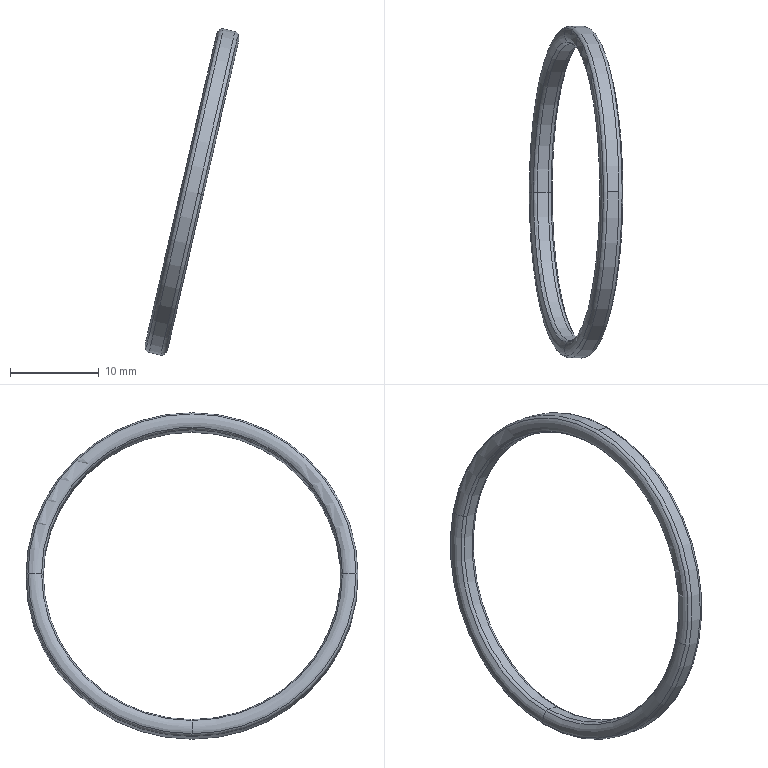Part | SolidWorks | features BaseBody 1 | 1 solid | 19 faces | box 10.587 x 37.5 x 36.875 mm | volume 507.842 mm3 | torus 15 | cylinder 4 | commonest cylinder face diameters 33.6 x2 37.5 x2
STEP:
#1=CARTESIAN_POINT('',(1987.878,-194.526,844.998));
#2=VERTEX_POINT('',#1);
#3=CARTESIAN_POINT('',(1983.731,-176.,826.943));
#4=VERTEX_POINT('',#3);
#5=CARTESIAN_POINT('',(1987.878,-176.,844.998));
#6=DIRECTION('',(0.9746,0.,-0.2239));
#7=DIRECTION('',(0.,-1.,0.));
#8=AXIS2_PLACEMENT_3D('',#5,#6,#7);
#9=CIRCLE('',#8,18.526);
#10=EDGE_CURVE('',#2,#4,#9,.T.);
#11=ORIENTED_EDGE('',*,*,#10,.F.);
#12=CARTESIAN_POINT('',(1987.472,-194.75,845.091));
#13=VERTEX_POINT('',#12);
#14=CARTESIAN_POINT('',(1987.472,-194.25,845.091));
#15=DIRECTION('',(-0.2239,0.,-0.9746));
#16=DIRECTION('',(-0.9746,0.,0.2239));
#17=AXIS2_PLACEMENT_3D('',#14,#15,#16);
#18=CIRCLE('',#17,0.5);
#19=EDGE_CURVE('',#2,#13,#18,.T.);
#20=ORIENTED_EDGE('',*,*,#19,.T.);
#21=CARTESIAN_POINT('',(1983.274,-176.,826.817));
#22=VERTEX_POINT('',#21);
#23=CARTESIAN_POINT('',(1987.472,-176.,845.091));
#24=DIRECTION('',(-0.9746,0.,0.2239));
#25=DIRECTION('',(-0.2239,0.,-0.9746));
#26=AXIS2_PLACEMENT_3D('',#23,#24,#25);
#27=CIRCLE('',#26,18.75);
#28=EDGE_CURVE('',#22,#13,#27,.T.);
#29=ORIENTED_EDGE('',*,*,#28,.F.);
#30=CARTESIAN_POINT('',(1983.386,-176.,827.305));
#31=DIRECTION('',(0.,-1.,0.));
#32=DIRECTION('',(0.6899,0.,-0.7239));
#33=AXIS2_PLACEMENT_3D('',#30,#31,#32);
#34=CIRCLE('',#33,0.5);
#35=EDGE_CURVE('',#22,#4,#34,.T.);
#36=ORIENTED_EDGE('',*,*,#35,.T.);
#37=EDGE_LOOP('',(#11,#20,#29,#36));
#38=FACE_OUTER_BOUND('',#37,.T.);
#39=CARTESIAN_POINT('',(1987.472,-176.,845.091));
#40=DIRECTION('',(-0.9746,0.,0.2239));
#41=DIRECTION('',(0.,-1.,0.));
#42=AXIS2_PLACEMENT_3D('',#39,#40,#41);
#43=TOROIDAL_SURFACE('',#42,18.25,0.5);
#44=ADVANCED_FACE('',(#38),#43,.T.);
#45=CARTESIAN_POINT('',(1987.809,-159.013,845.014));
#46=VERTEX_POINT('',#45);
#47=CARTESIAN_POINT('',(1984.007,-176.,828.458));
#48=VERTEX_POINT('',#47);
#49=CARTESIAN_POINT('',(1987.809,-176.,845.014));
#50=DIRECTION('',(-0.9746,0.,0.2239));
#51=DIRECTION('',(0.,1.,0.));
#52=AXIS2_PLACEMENT_3D('',#49,#50,#51);
#53=CIRCLE('',#52,16.987);
#54=EDGE_CURVE('',#46,#48,#53,.T.);
#55=ORIENTED_EDGE('',*,*,#54,.T.);
#56=CARTESIAN_POINT('',(1982.829,-176.,827.889));
#57=DIRECTION('',(0.,1.,0.));
#58=DIRECTION('',(0.,0.,1.));
#59=AXIS2_PLACEMENT_3D('',#56,#57,#58);
#60=CIRCLE('',#59,1.308);
#61=EDGE_CURVE('',#48,#4,#60,.T.);
#62=ORIENTED_EDGE('',*,*,#61,.T.);
#63=CARTESIAN_POINT('',(1987.878,-157.474,844.998));
#64=VERTEX_POINT('',#63);
#65=CARTESIAN_POINT('',(1987.878,-176.,844.998));
#66=DIRECTION('',(0.9746,0.,-0.2239));
#67=DIRECTION('',(-0.2239,0.,-0.9746));
#68=AXIS2_PLACEMENT_3D('',#65,#66,#67);
#69=CIRCLE('',#68,18.526);
#70=EDGE_CURVE('',#4,#64,#69,.T.);
#71=ORIENTED_EDGE('',*,*,#70,.T.);
#72=CARTESIAN_POINT('',(1986.815,-158.195,845.242));
#73=DIRECTION('',(0.2239,0.,0.9746));
#74=DIRECTION('',(0.7605,-0.6254,-0.1747));
#75=AXIS2_PLACEMENT_3D('',#72,#73,#74);
#76=CIRCLE('',#75,1.307);
#77=EDGE_CURVE('',#46,#64,#76,.T.);
#78=ORIENTED_EDGE('',*,*,#77,.F.);
#79=EDGE_LOOP('',(#55,#62,#71,#78));
#80=FACE_OUTER_BOUND('',#79,.T.);
#81=CARTESIAN_POINT('',(1986.815,-176.,845.242));
#82=DIRECTION('',(-0.9746,0.,0.2239));
#83=DIRECTION('',(-0.2239,0.,-0.9746));
#84=AXIS2_PLACEMENT_3D('',#81,#82,#83);
#85=TOROIDAL_SURFACE('',#84,17.805,1.308);
#86=ADVANCED_FACE('',(#80),#85,.T.);
#87=CARTESIAN_POINT('',(1985.752,-157.474,845.486));
#88=VERTEX_POINT('',#87);
#89=CARTESIAN_POINT('',(1981.604,-176.,827.431));
#90=VERTEX_POINT('',#89);
#91=CARTESIAN_POINT('',(1985.752,-176.,845.486));
#92=DIRECTION('',(-0.9746,0.,0.2239));
#93=DIRECTION('',(0.,1.,0.));
#94=AXIS2_PLACEMENT_3D('',#91,#92,#93);
#95=CIRCLE('',#94,18.526);
#96=EDGE_CURVE('',#88,#90,#95,.T.);
#97=ORIENTED_EDGE('',*,*,#96,.T.);
#98=CARTESIAN_POINT('',(1982.018,-176.,828.914));
#99=VERTEX_POINT('',#98);
#100=CARTESIAN_POINT('',(1982.829,-176.,827.889));
#101=DIRECTION('',(0.,1.,0.));
#102=DIRECTION('',(0.,0.,1.));
#103=AXIS2_PLACEMENT_3D('',#100,#101,#102);
#104=CIRCLE('',#103,1.308);
#105=EDGE_CURVE('',#90,#99,#104,.T.);
#106=ORIENTED_EDGE('',*,*,#105,.T.);
#107=CARTESIAN_POINT('',(1985.821,-159.013,845.471));
#108=VERTEX_POINT('',#107);
#109=CARTESIAN_POINT('',(1985.821,-176.,845.471));
#110=DIRECTION('',(0.9746,0.,-0.2239));
#111=DIRECTION('',(-0.2239,0.,-0.9746));
#112=AXIS2_PLACEMENT_3D('',#109,#110,#111);
#113=CIRCLE('',#112,16.987);
#114=EDGE_CURVE('',#99,#108,#113,.T.);
#115=ORIENTED_EDGE('',*,*,#114,.T.);
#116=CARTESIAN_POINT('',(1986.815,-158.195,845.242));
#117=DIRECTION('',(0.2239,0.,0.9746));
#118=DIRECTION('',(-0.8133,0.5511,0.1868));
#119=AXIS2_PLACEMENT_3D('',#116,#117,#118);
#120=CIRCLE('',#119,1.308);
#121=EDGE_CURVE('',#88,#108,#120,.T.);
#122=ORIENTED_EDGE('',*,*,#121,.F.);
#123=EDGE_LOOP('',(#97,#106,#115,#122));
#124=FACE_OUTER_BOUND('',#123,.T.);
#125=CARTESIAN_POINT('',(1986.815,-176.,845.242));
#126=DIRECTION('',(-0.9746,0.,0.2239));
#127=DIRECTION('',(-0.2239,0.,-0.9746));
#128=AXIS2_PLACEMENT_3D('',#125,#126,#127);
#129=TOROIDAL_SURFACE('',#128,17.805,1.308);
#130=ADVANCED_FACE('',(#124),#129,.T.);
#131=ORIENTED_EDGE('',*,*,#121,.T.);
#132=CARTESIAN_POINT('',(1985.821,-192.987,845.471));
#133=VERTEX_POINT('',#132);
#134=CARTESIAN_POINT('',(1985.821,-176.,845.471));
#135=DIRECTION('',(0.9746,0.,-0.2239));
#136=DIRECTION('',(0.,1.,0.));
#137=AXIS2_PLACEMENT_3D('',#134,#135,#136);
#138=CIRCLE('',#137,16.987);
#139=EDGE_CURVE('',#108,#133,#138,.T.);
#140=ORIENTED_EDGE('',*,*,#139,.T.);
#141=CARTESIAN_POINT('',(1985.752,-194.526,845.486));
#142=VERTEX_POINT('',#141);
#143=CARTESIAN_POINT('',(1986.815,-193.805,845.242));
#144=DIRECTION('',(0.2239,0.,0.9746));
#145=DIRECTION('',(-0.7605,0.6254,0.1747));
#146=AXIS2_PLACEMENT_3D('',#143,#144,#145);
#147=CIRCLE('',#146,1.307);
#148=EDGE_CURVE('',#133,#142,#147,.T.);
#149=ORIENTED_EDGE('',*,*,#148,.T.);
#150=CARTESIAN_POINT('',(1985.752,-176.,845.486));
#151=DIRECTION('',(-0.9746,0.,0.2239));
#152=DIRECTION('',(0.000000025,-1.,0.00000011));
#153=AXIS2_PLACEMENT_3D('',#150,#151,#152);
#154=CIRCLE('',#153,18.526);
#155=EDGE_CURVE('',#142,#88,#154,.T.);
#156=ORIENTED_EDGE('',*,*,#155,.T.);
#157=EDGE_LOOP('',(#131,#140,#149,#156));
#158=FACE_OUTER_BOUND('',#157,.T.);
#159=CARTESIAN_POINT('',(1986.815,-176.,845.242));
#160=DIRECTION('',(-0.9746,0.,0.2239));
#161=DIRECTION('',(-0.2239,0.,-0.9746));
#162=AXIS2_PLACEMENT_3D('',#159,#160,#161);
#163=TOROIDAL_SURFACE('',#162,17.805,1.308);
#164=ADVANCED_FACE('',(#158),#163,.T.);
#165=CARTESIAN_POINT('',(1987.809,-192.987,845.014));
#166=VERTEX_POINT('',#165);
#167=CARTESIAN_POINT('',(1986.815,-193.805,845.242));
#168=DIRECTION('',(0.2239,0.,0.9746));
#169=DIRECTION('',(0.8133,-0.5511,-0.1868));
#170=AXIS2_PLACEMENT_3D('',#167,#168,#169);
#171=CIRCLE('',#170,1.308);
#172=EDGE_CURVE('',#2,#166,#171,.T.);
#173=ORIENTED_EDGE('',*,*,#172,.T.);
#174=CARTESIAN_POINT('',(1987.809,-176.,845.014));
#175=DIRECTION('',(-0.9746,0.,0.2239));
#176=DIRECTION('',(-0.000000032,-1.,-0.000000138));
#177=AXIS2_PLACEMENT_3D('',#174,#175,#176);
#178=CIRCLE('',#177,16.987);
#179=EDGE_CURVE('',#166,#46,#178,.T.);
#180=ORIENTED_EDGE('',*,*,#179,.T.);
#181=ORIENTED_EDGE('',*,*,#77,.T.);
#182=CARTESIAN_POINT('',(1987.878,-176.,844.998));
#183=DIRECTION('',(0.9746,0.,-0.2239));
#184=DIRECTION('',(0.,1.,0.));
#185=AXIS2_PLACEMENT_3D('',#182,#183,#184);
#186=CIRCLE('',#185,18.526);
#187=EDGE_CURVE('',#64,#2,#186,.T.);
#188=ORIENTED_EDGE('',*,*,#187,.T.);
#189=EDGE_LOOP('',(#173,#180,#181,#188));
#190=FACE_OUTER_BOUND('',#189,.T.);
#191=CARTESIAN_POINT('',(1986.815,-176.,845.242));
#192=DIRECTION('',(-0.9746,0.,0.2239));
#193=DIRECTION('',(-0.2239,0.,-0.9746));
#194=AXIS2_PLACEMENT_3D('',#191,#192,#193);
#195=TOROIDAL_SURFACE('',#194,17.805,1.308);
#196=ADVANCED_FACE('',(#190),#195,.T.);
#197=CARTESIAN_POINT('',(1985.752,-176.,845.486));
#198=DIRECTION('',(-0.9746,0.,0.2239));
#199=DIRECTION('',(-0.2239,0.,-0.9746));
#200=AXIS2_PLACEMENT_3D('',#197,#198,#199);
#201=CIRCLE('',#200,18.526);
#202=EDGE_CURVE('',#90,#142,#201,.T.);
#203=ORIENTED_EDGE('',*,*,#202,.F.);
#204=CARTESIAN_POINT('',(1981.961,-176.,827.119));
#205=VERTEX_POINT('',#204);
#206=CARTESIAN_POINT('',(1982.073,-176.,827.606));
#207=DIRECTION('',(0.,-1.,0.));
#208=DIRECTION('',(-0.9366,0.,-0.3503));
#209=AXIS2_PLACEMENT_3D('',#206,#207,#208);
#210=CIRCLE('',#209,0.5);
#211=EDGE_CURVE('',#90,#205,#210,.T.);
#212=ORIENTED_EDGE('',*,*,#211,.T.);
#213=CARTESIAN_POINT('',(1990.356,-176.,863.667));
#214=VERTEX_POINT('',#213);
#215=CARTESIAN_POINT('',(1986.158,-176.,845.393));
#216=DIRECTION('',(0.9746,0.,-0.2239));
#217=DIRECTION('',(0.2239,0.,0.9746));
#218=AXIS2_PLACEMENT_3D('',#215,#216,#217);
#219=CIRCLE('',#218,18.75);
#220=EDGE_CURVE('',#214,#205,#219,.T.);
#221=ORIENTED_EDGE('',*,*,#220,.F.);
#222=CARTESIAN_POINT('',(1986.158,-157.25,845.393));
#223=VERTEX_POINT('',#222);
#224=CARTESIAN_POINT('',(1986.158,-176.,845.393));
#225=DIRECTION('',(-0.9746,0.,0.2239));
#226=DIRECTION('',(0.2239,0.,0.9746));
#227=AXIS2_PLACEMENT_3D('',#224,#225,#226);
#228=CIRCLE('',#227,18.75);
#229=EDGE_CURVE('',#214,#223,#228,.T.);
#230=ORIENTED_EDGE('',*,*,#229,.T.);
#231=CARTESIAN_POINT('',(1986.158,-157.75,845.393));
#232=DIRECTION('',(0.2239,0.,0.9746));
#233=DIRECTION('',(-0.8133,0.5511,0.1868));
#234=AXIS2_PLACEMENT_3D('',#231,#232,#233);
#235=CIRCLE('',#234,0.5);
#236=EDGE_CURVE('',#223,#88,#235,.T.);
#237=ORIENTED_EDGE('',*,*,#236,.T.);
#238=ORIENTED_EDGE('',*,*,#155,.F.);
#239=EDGE_LOOP('',(#203,#212,#221,#230,#237,#238));
#240=FACE_OUTER_BOUND('',#239,.T.);
#241=CARTESIAN_POINT('',(1986.158,-176.,845.393));
#242=DIRECTION('',(-0.9746,0.,0.2239));
#243=DIRECTION('',(-0.2239,0.,-0.9746));
#244=AXIS2_PLACEMENT_3D('',#241,#242,#243);
#245=TOROIDAL_SURFACE('',#244,18.25,0.5);
#246=ADVANCED_FACE('',(#240),#245,.T.);
#247=ORIENTED_EDGE('',*,*,#236,.F.);
#248=CARTESIAN_POINT('',(1986.158,-176.,845.393));
#249=DIRECTION('',(-0.9746,0.,0.2239));
#250=DIRECTION('',(0.,1.,0.));
#251=AXIS2_PLACEMENT_3D('',#248,#249,#250);
#252=CIRCLE('',#251,18.75);
#253=EDGE_CURVE('',#223,#205,#252,.T.);
#254=ORIENTED_EDGE('',*,*,#253,.T.);
#255=ORIENTED_EDGE('',*,*,#211,.F.);
#256=ORIENTED_EDGE('',*,*,#96,.F.);
#257=EDGE_LOOP('',(#247,#254,#255,#256));
#258=FACE_OUTER_BOUND('',#257,.T.);
#259=CARTESIAN_POINT('',(1986.158,-176.,845.393));
#260=DIRECTION('',(-0.9746,0.,0.2239));
#261=DIRECTION('',(-0.2239,0.,-0.9746));
#262=AXIS2_PLACEMENT_3D('',#259,#260,#261);
#263=TOROIDAL_SURFACE('',#262,18.25,0.5);
#264=ADVANCED_FACE('',(#258),#263,.T.);
#265=ORIENTED_EDGE('',*,*,#105,.F.);
#266=ORIENTED_EDGE('',*,*,#202,.T.);
#267=ORIENTED_EDGE('',*,*,#148,.F.);
#268=CARTESIAN_POINT('',(1985.821,-176.,845.471));
#269=DIRECTION('',(0.9746,0.,-0.2239));
#270=DIRECTION('',(0.,-1.,0.));
#271=AXIS2_PLACEMENT_3D('',#268,#269,#270);
#272=CIRCLE('',#271,16.987);
#273=EDGE_CURVE('',#133,#99,#272,.T.);
#274=ORIENTED_EDGE('',*,*,#273,.T.);
#275=EDGE_LOOP('',(#265,#266,#267,#274));
#276=FACE_OUTER_BOUND('',#275,.T.);
#277=CARTESIAN_POINT('',(1986.815,-176.,845.242));
#278=DIRECTION('',(-0.9746,0.,0.2239));
#279=DIRECTION('',(-0.2239,0.,-0.9746));
#280=AXIS2_PLACEMENT_3D('',#277,#278,#279);
#281=TOROIDAL_SURFACE('',#280,17.805,1.308);
#282=ADVANCED_FACE('',(#276),#281,.T.);
#283=ORIENTED_EDGE('',*,*,#61,.F.);
#284=CARTESIAN_POINT('',(1987.809,-176.,845.014));
#285=DIRECTION('',(-0.9746,0.,0.2239));
#286=DIRECTION('',(-0.2239,0.,-0.9746));
#287=AXIS2_PLACEMENT_3D('',#284,#285,#286);
#288=CIRCLE('',#287,16.987);
#289=EDGE_CURVE('',#48,#166,#288,.T.);
#290=ORIENTED_EDGE('',*,*,#289,.T.);
#291=ORIENTED_EDGE('',*,*,#172,.F.);
#292=ORIENTED_EDGE('',*,*,#10,.T.);
#293=EDGE_LOOP('',(#283,#290,#291,#292));
#294=FACE_OUTER_BOUND('',#293,.T.);
#295=CARTESIAN_POINT('',(1986.815,-176.,845.242));
#296=DIRECTION('',(-0.9746,0.,0.2239));
#297=DIRECTION('',(-0.2239,0.,-0.9746));
#298=AXIS2_PLACEMENT_3D('',#295,#296,#297);
#299=TOROIDAL_SURFACE('',#298,17.805,1.308);
#300=ADVANCED_FACE('',(#294),#299,.T.);
#301=CARTESIAN_POINT('',(1982.44,-176.,829.01));
#302=VERTEX_POINT('',#301);
#303=CARTESIAN_POINT('',(1982.328,-176.,828.522));
#304=DIRECTION('',(0.,1.,0.));
#305=DIRECTION('',(-0.6205,0.,0.7842));
#306=AXIS2_PLACEMENT_3D('',#303,#304,#305);
#307=CIRCLE('',#306,0.5);
#308=EDGE_CURVE('',#99,#302,#307,.T.);
#309=ORIENTED_EDGE('',*,*,#308,.T.);
#310=CARTESIAN_POINT('',(1986.201,-159.2,845.383));
#311=VERTEX_POINT('',#310);
#312=CARTESIAN_POINT('',(1986.201,-176.,845.383));
#313=DIRECTION('',(0.9746,0.,-0.2239));
#314=DIRECTION('',(-0.2239,0.,-0.9746));
#315=AXIS2_PLACEMENT_3D('',#312,#313,#314);
#316=CIRCLE('',#315,16.8);
#317=EDGE_CURVE('',#302,#311,#316,.T.);
#318=ORIENTED_EDGE('',*,*,#317,.T.);
#319=CARTESIAN_POINT('',(1986.201,-158.7,845.383));
#320=DIRECTION('',(-0.2239,0.,-0.9746));
#321=DIRECTION('',(-0.7605,-0.6254,0.1747));
#322=AXIS2_PLACEMENT_3D('',#319,#320,#321);
#323=CIRCLE('',#322,0.5);
#324=EDGE_CURVE('',#311,#108,#323,.T.);
#325=ORIENTED_EDGE('',*,*,#324,.T.);
#326=ORIENTED_EDGE('',*,*,#114,.F.);
#327=EDGE_LOOP('',(#309,#318,#325,#326));
#328=FACE_OUTER_BOUND('',#327,.T.);
#329=CARTESIAN_POINT('',(1986.201,-176.,845.383));
#330=DIRECTION('',(-0.9746,0.,0.2239));
#331=DIRECTION('',(-0.2239,0.,-0.9746));
#332=AXIS2_PLACEMENT_3D('',#329,#330,#331);
#333=TOROIDAL_SURFACE('',#332,17.3,0.5);
#334=ADVANCED_FACE('',(#328),#333,.T.);
#335=ORIENTED_EDGE('',*,*,#324,.F.);
#336=CARTESIAN_POINT('',(1989.962,-176.,861.757));
#337=VERTEX_POINT('',#336);
#338=CARTESIAN_POINT('',(1986.201,-176.,845.383));
#339=DIRECTION('',(0.9746,0.,-0.2239));
#340=DIRECTION('',(0.,1.,0.));
#341=AXIS2_PLACEMENT_3D('',#338,#339,#340);
#342=CIRCLE('',#341,16.8);
#343=EDGE_CURVE('',#311,#337,#342,.T.);
#344=ORIENTED_EDGE('',*,*,#343,.T.);
#345=CARTESIAN_POINT('',(1986.201,-176.,845.383));
#346=DIRECTION('',(-0.9746,0.,0.2239));
#347=DIRECTION('',(-0.2239,0.,-0.9746));
#348=AXIS2_PLACEMENT_3D('',#345,#346,#347);
#349=CIRCLE('',#348,16.8);
#350=EDGE_CURVE('',#302,#337,#349,.T.);
#351=ORIENTED_EDGE('',*,*,#350,.F.);
#352=ORIENTED_EDGE('',*,*,#308,.F.);
#353=ORIENTED_EDGE('',*,*,#273,.F.);
#354=ORIENTED_EDGE('',*,*,#139,.F.);
#355=EDGE_LOOP('',(#335,#344,#351,#352,#353,#354));
#356=FACE_OUTER_BOUND('',#355,.T.);
#357=CARTESIAN_POINT('',(1986.201,-176.,845.383));
#358=DIRECTION('',(-0.9746,0.,0.2239));
#359=DIRECTION('',(-0.2239,0.,-0.9746));
#360=AXIS2_PLACEMENT_3D('',#357,#358,#359);
#361=TOROIDAL_SURFACE('',#360,17.3,0.5);
#362=ADVANCED_FACE('',(#356),#361,.T.);
#363=CARTESIAN_POINT('',(1991.19,-176.,861.475));
#364=VERTEX_POINT('',#363);
#365=CARTESIAN_POINT('',(1989.962,-176.,861.757));
#366=DIRECTION('',(0.9746,0.,-0.2239));
#367=VECTOR('',#366,1000.);
#368=LINE('',#365,#367);
#369=EDGE_CURVE('',#337,#364,#368,.T.);
#370=ORIENTED_EDGE('',*,*,#369,.T.);
#371=CARTESIAN_POINT('',(1983.668,-176.,828.728));
#372=VERTEX_POINT('',#371);
#373=CARTESIAN_POINT('',(1987.429,-176.,845.101));
#374=DIRECTION('',(0.9746,0.,-0.2239));
#375=DIRECTION('',(0.2239,0.,0.9746));
#376=AXIS2_PLACEMENT_3D('',#373,#374,#375);
#377=CIRCLE('',#376,16.8);
#378=EDGE_CURVE('',#364,#372,#377,.T.);
#379=ORIENTED_EDGE('',*,*,#378,.T.);
#380=CARTESIAN_POINT('',(1982.44,-176.,829.01));
#381=DIRECTION('',(-0.9746,0.,0.2239));
#382=VECTOR('',#381,1000.);
#383=LINE('',#380,#382);
#384=EDGE_CURVE('',#372,#302,#383,.T.);
#385=ORIENTED_EDGE('',*,*,#384,.T.);
#386=ORIENTED_EDGE('',*,*,#350,.T.);
#387=EDGE_LOOP('',(#370,#379,#385,#386));
#388=FACE_OUTER_BOUND('',#387,.T.);
#389=CARTESIAN_POINT('',(1987.546,-176.,845.074));
#390=DIRECTION('',(-0.9746,0.,0.2239));
#391=DIRECTION('',(-0.2239,0.,-0.9746));
#392=AXIS2_PLACEMENT_3D('',#389,#390,#391);
#393=CYLINDRICAL_SURFACE('',#392,16.8);
#394=ADVANCED_FACE('',(#388),#393,.F.);
#395=ORIENTED_EDGE('',*,*,#384,.F.);
#396=CARTESIAN_POINT('',(1987.429,-159.2,845.101));
#397=VERTEX_POINT('',#396);
#398=CARTESIAN_POINT('',(1987.429,-176.,845.101));
#399=DIRECTION('',(-0.9746,0.,0.2239));
#400=DIRECTION('',(0.,1.,0.));
#401=AXIS2_PLACEMENT_3D('',#398,#399,#400);
#402=CIRCLE('',#401,16.8);
#403=EDGE_CURVE('',#397,#372,#402,.T.);
#404=ORIENTED_EDGE('',*,*,#403,.F.);
#405=CARTESIAN_POINT('',(1987.429,-176.,845.101));
#406=DIRECTION('',(-0.9746,0.,0.2239));
#407=DIRECTION('',(0.2239,0.,0.9746));
#408=AXIS2_PLACEMENT_3D('',#405,#406,#407);
#409=CIRCLE('',#408,16.8);
#410=EDGE_CURVE('',#364,#397,#409,.T.);
#411=ORIENTED_EDGE('',*,*,#410,.F.);
#412=ORIENTED_EDGE('',*,*,#369,.F.);
#413=ORIENTED_EDGE('',*,*,#343,.F.);
#414=ORIENTED_EDGE('',*,*,#317,.F.);
#415=EDGE_LOOP('',(#395,#404,#411,#412,#413,#414));
#416=FACE_OUTER_BOUND('',#415,.T.);
#417=CARTESIAN_POINT('',(1987.546,-176.,845.074));
#418=DIRECTION('',(-0.9746,0.,0.2239));
#419=DIRECTION('',(-0.2239,0.,-0.9746));
#420=AXIS2_PLACEMENT_3D('',#417,#418,#419);
#421=CYLINDRICAL_SURFACE('',#420,16.8);
#422=ADVANCED_FACE('',(#416),#421,.F.);
#423=ORIENTED_EDGE('',*,*,#289,.F.);
#424=CARTESIAN_POINT('',(1983.556,-176.,828.24));
#425=DIRECTION('',(0.,1.,0.));
#426=DIRECTION('',(0.9005,0.,0.4348));
#427=AXIS2_PLACEMENT_3D('',#424,#425,#426);
#428=CIRCLE('',#427,0.5);
#429=EDGE_CURVE('',#372,#48,#428,.T.);
#430=ORIENTED_EDGE('',*,*,#429,.F.);
#431=ORIENTED_EDGE('',*,*,#378,.F.);
#432=ORIENTED_EDGE('',*,*,#410,.T.);
#433=CARTESIAN_POINT('',(1987.429,-158.7,845.101));
#434=DIRECTION('',(-0.2239,0.,-0.9746));
#435=DIRECTION('',(0.7605,-0.6254,-0.1747));
#436=AXIS2_PLACEMENT_3D('',#433,#434,#435);
#437=CIRCLE('',#436,0.5);
#438=EDGE_CURVE('',#46,#397,#437,.T.);
#439=ORIENTED_EDGE('',*,*,#438,.F.);
#440=ORIENTED_EDGE('',*,*,#179,.F.);
#441=EDGE_LOOP('',(#423,#430,#431,#432,#439,#440));
#442=FACE_OUTER_BOUND('',#441,.T.);
#443=CARTESIAN_POINT('',(1987.429,-176.,845.101));
#444=DIRECTION('',(-0.9746,0.,0.2239));
#445=DIRECTION('',(-0.2239,0.,-0.9746));
#446=AXIS2_PLACEMENT_3D('',#443,#444,#445);
#447=TOROIDAL_SURFACE('',#446,17.3,0.5);
#448=ADVANCED_FACE('',(#442),#447,.T.);
#449=ORIENTED_EDGE('',*,*,#438,.T.);
#450=ORIENTED_EDGE('',*,*,#403,.T.);
#451=ORIENTED_EDGE('',*,*,#429,.T.);
#452=ORIENTED_EDGE('',*,*,#54,.F.);
#453=EDGE_LOOP('',(#449,#450,#451,#452));
#454=FACE_OUTER_BOUND('',#453,.T.);
#455=CARTESIAN_POINT('',(1987.429,-176.,845.101));
#456=DIRECTION('',(-0.9746,0.,0.2239));
#457=DIRECTION('',(-0.2239,0.,-0.9746));
#458=AXIS2_PLACEMENT_3D('',#455,#456,#457);
#459=TOROIDAL_SURFACE('',#458,17.3,0.5);
#460=ADVANCED_FACE('',(#454),#459,.T.);
#461=ORIENTED_EDGE('',*,*,#19,.F.);
#462=ORIENTED_EDGE('',*,*,#187,.F.);
#463=CARTESIAN_POINT('',(1987.472,-157.25,845.091));
#464=VERTEX_POINT('',#463);
#465=CARTESIAN_POINT('',(1987.472,-157.75,845.091));
#466=DIRECTION('',(0.2239,0.,0.9746));
#467=DIRECTION('',(0.8133,0.5511,-0.1868));
#468=AXIS2_PLACEMENT_3D('',#465,#466,#467);
#469=CIRCLE('',#468,0.5);
#470=EDGE_CURVE('',#64,#464,#469,.T.);
#471=ORIENTED_EDGE('',*,*,#470,.T.);
#472=CARTESIAN_POINT('',(1991.669,-176.,863.365));
#473=VERTEX_POINT('',#472);
#474=CARTESIAN_POINT('',(1987.472,-176.,845.091));
#475=DIRECTION('',(0.9746,0.,-0.2239));
#476=DIRECTION('',(-0.000000003,1.,-0.000000014));
#477=AXIS2_PLACEMENT_3D('',#474,#475,#476);
#478=CIRCLE('',#477,18.75);
#479=EDGE_CURVE('',#464,#473,#478,.T.);
#480=ORIENTED_EDGE('',*,*,#479,.T.);
#481=CARTESIAN_POINT('',(1987.472,-176.,845.091));
#482=DIRECTION('',(-0.9746,0.,0.2239));
#483=DIRECTION('',(-0.2239,0.,-0.9746));
#484=AXIS2_PLACEMENT_3D('',#481,#482,#483);
#485=CIRCLE('',#484,18.75);
#486=EDGE_CURVE('',#13,#473,#485,.T.);
#487=ORIENTED_EDGE('',*,*,#486,.F.);
#488=EDGE_LOOP('',(#461,#462,#471,#480,#487));
#489=FACE_OUTER_BOUND('',#488,.T.);
#490=CARTESIAN_POINT('',(1987.472,-176.,845.091));
#491=DIRECTION('',(-0.9746,0.,0.2239));
#492=DIRECTION('',(0.,-1.,0.));
#493=AXIS2_PLACEMENT_3D('',#490,#491,#492);
#494=TOROIDAL_SURFACE('',#493,18.25,0.5);
#495=ADVANCED_FACE('',(#489),#494,.T.);
#496=ORIENTED_EDGE('',*,*,#35,.F.);
#497=CARTESIAN_POINT('',(1987.472,-176.,845.091));
#498=DIRECTION('',(0.9746,0.,-0.2239));
#499=DIRECTION('',(-0.2239,0.,-0.9746));
#500=AXIS2_PLACEMENT_3D('',#497,#498,#499);
#501=CIRCLE('',#500,18.75);
#502=EDGE_CURVE('',#22,#464,#501,.T.);
#503=ORIENTED_EDGE('',*,*,#502,.T.);
#504=ORIENTED_EDGE('',*,*,#470,.F.);
#505=ORIENTED_EDGE('',*,*,#70,.F.);
#506=EDGE_LOOP('',(#496,#503,#504,#505));
#507=FACE_OUTER_BOUND('',#506,.T.);
#508=CARTESIAN_POINT('',(1987.472,-176.,845.091));
#509=DIRECTION('',(-0.9746,0.,0.2239));
#510=DIRECTION('',(-0.2239,0.,-0.9746));
#511=AXIS2_PLACEMENT_3D('',#508,#509,#510);
#512=TOROIDAL_SURFACE('',#511,18.25,0.5);
#513=ADVANCED_FACE('',(#507),#512,.T.);
#514=CARTESIAN_POINT('',(1990.356,-176.,863.667));
#515=DIRECTION('',(0.9746,0.,-0.2239));
#516=VECTOR('',#515,1000.);
#517=LINE('',#514,#516);
#518=EDGE_CURVE('',#214,#473,#517,.T.);
#519=ORIENTED_EDGE('',*,*,#518,.T.);
#520=ORIENTED_EDGE('',*,*,#479,.F.);
#521=ORIENTED_EDGE('',*,*,#502,.F.);
#522=CARTESIAN_POINT('',(1981.961,-176.,827.119));
#523=DIRECTION('',(-0.9746,0.,0.2239));
#524=VECTOR('',#523,1000.);
#525=LINE('',#522,#524);
#526=EDGE_CURVE('',#22,#205,#525,.T.);
#527=ORIENTED_EDGE('',*,*,#526,.T.);
#528=ORIENTED_EDGE('',*,*,#253,.F.);
#529=ORIENTED_EDGE('',*,*,#229,.F.);
#530=EDGE_LOOP('',(#519,#520,#521,#527,#528,#529));
#531=FACE_OUTER_BOUND('',#530,.T.);
#532=CARTESIAN_POINT('',(1987.589,-176.,845.064));
#533=DIRECTION('',(-0.9746,0.,0.2239));
#534=DIRECTION('',(-0.2239,0.,-0.9746));
#535=AXIS2_PLACEMENT_3D('',#532,#533,#534);
#536=CYLINDRICAL_SURFACE('',#535,18.75);
#537=ADVANCED_FACE('',(#531),#536,.T.);
#538=ORIENTED_EDGE('',*,*,#526,.F.);
#539=ORIENTED_EDGE('',*,*,#28,.T.);
#540=ORIENTED_EDGE('',*,*,#486,.T.);
#541=ORIENTED_EDGE('',*,*,#518,.F.);
#542=ORIENTED_EDGE('',*,*,#220,.T.);
#543=EDGE_LOOP('',(#538,#539,#540,#541,#542));
#544=FACE_OUTER_BOUND('',#543,.T.);
#545=CARTESIAN_POINT('',(1987.589,-176.,845.064));
#546=DIRECTION('',(-0.9746,0.,0.2239));
#547=DIRECTION('',(-0.2239,0.,-0.9746));
#548=AXIS2_PLACEMENT_3D('',#545,#546,#547);
#549=CYLINDRICAL_SURFACE('',#548,18.75);
#550=ADVANCED_FACE('',(#544),#549,.T.);
#551=CLOSED_SHELL('',(#44,#86,#130,#164,#196,#246,#264,#282,#300,#334,#362,#394,#422,#448,#460,#495,#513,#537,#550));
#552=MANIFOLD_SOLID_BREP('',#551);
#553=CARTESIAN_POINT('',(0.,0.,0.));
#554=DIRECTION('',(0.,0.,1.));
#555=DIRECTION('',(1.,0.,0.));
#556=AXIS2_PLACEMENT_3D('',#553,#554,#555);
#557=(LENGTH_UNIT()NAMED_UNIT(*)SI_UNIT(.MILLI.,.METRE.));
#558=UNCERTAINTY_MEASURE_WITH_UNIT(LENGTH_MEASURE(0.00001),#557,'','');
#559=(NAMED_UNIT(*)PLANE_ANGLE_UNIT()SI_UNIT($,.RADIAN.));
#560=(NAMED_UNIT(*)SI_UNIT($,.STERADIAN.)SOLID_ANGLE_UNIT());
#561=(GEOMETRIC_REPRESENTATION_CONTEXT(3)GLOBAL_UNCERTAINTY_ASSIGNED_CONTEXT((#558))GLOBAL_UNIT_ASSIGNED_CONTEXT((#557,#559,#560))REPRESENTATION_CONTEXT('',''));
#562=ADVANCED_BREP_SHAPE_REPRESENTATION('',(#552,#556),#561);